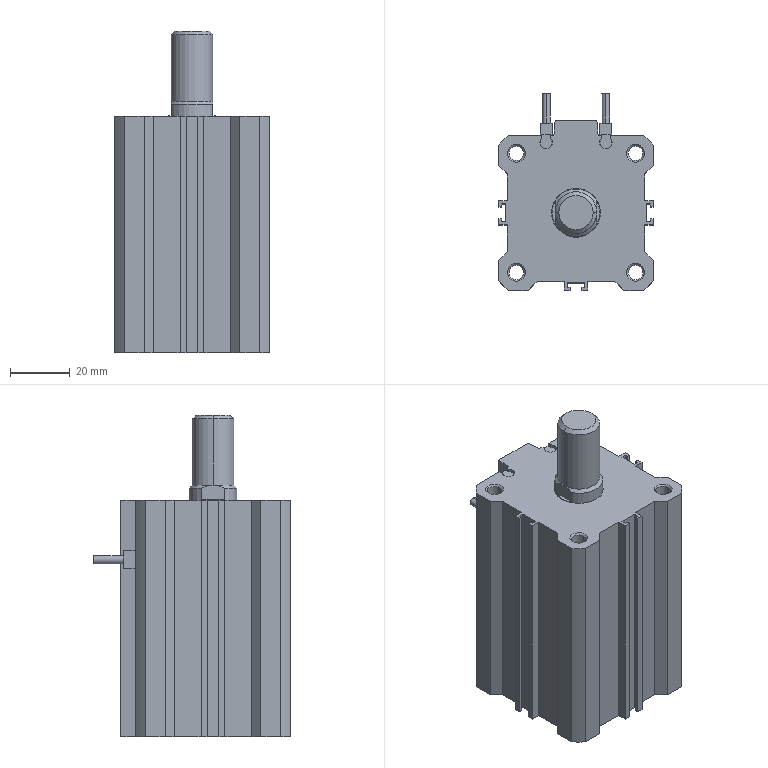Part | STEP file | A_CDQ2A40-40DM-A96V(0) | 2 solids | 163 faces | box 52 x 66.1 x 108 mm | volume 193246 mm3 | plane 93 | cylinder 38 | cone 24 | spline 8 | commonest cylinder face diameters 4.92 x8 4 x6 4.2 x6 2.7 x4 8.57 x4 69 x4